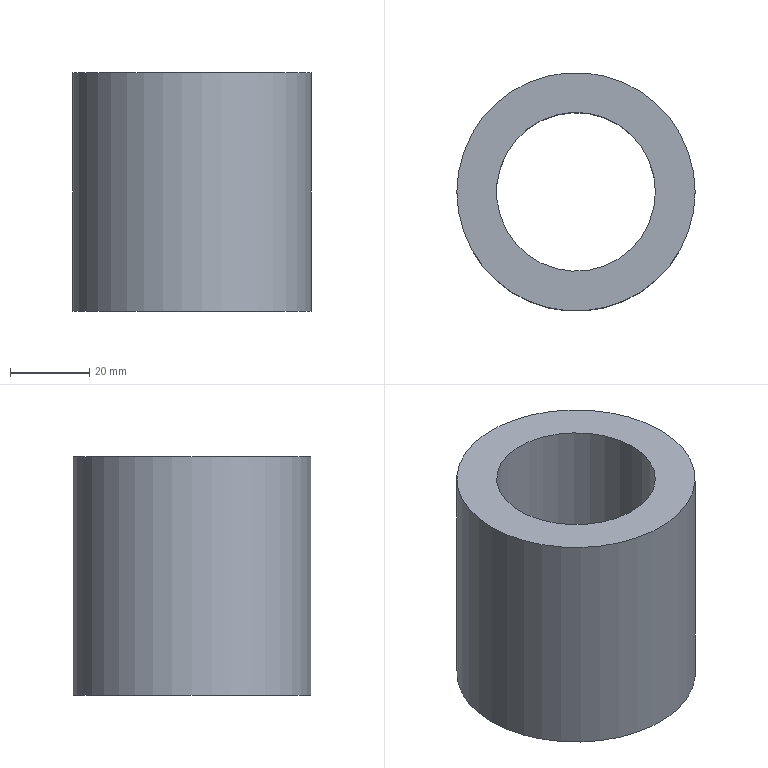Part | NX | features solid 2 | 1 solid | 4 faces | box 60 x 60 x 60 mm | volume 94248 mm3 | cylinder 2 | plane 2 | commonest cylinder face diameters 40 x1 60 x1
STEP:
#1=CARTESIAN_POINT('',(215.,25.,30.));
#2=VERTEX_POINT('',#1);
#3=CARTESIAN_POINT('',(195.,25.,30.));
#4=DIRECTION('',(0.,0.,-1.));
#5=DIRECTION('',(1.,0.,0.));
#6=AXIS2_PLACEMENT_3D('',#3,#4,#5);
#7=CIRCLE('',#6,20.);
#8=EDGE_CURVE('',#2,#2,#7,.T.);
#9=ORIENTED_EDGE('',*,*,#8,.T.);
#10=EDGE_LOOP('',(#9));
#11=FACE_BOUND('',#10,.T.);
#12=CARTESIAN_POINT('',(215.,25.,90.));
#13=VERTEX_POINT('',#12);
#14=CARTESIAN_POINT('',(195.,25.,90.));
#15=DIRECTION('',(0.,0.,-1.));
#16=DIRECTION('',(1.,0.,0.));
#17=AXIS2_PLACEMENT_3D('',#14,#15,#16);
#18=CIRCLE('',#17,20.);
#19=EDGE_CURVE('',#13,#13,#18,.T.);
#20=ORIENTED_EDGE('',*,*,#19,.F.);
#21=EDGE_LOOP('',(#20));
#22=FACE_BOUND('',#21,.T.);
#23=CARTESIAN_POINT('',(195.,25.,30.));
#24=DIRECTION('',(0.,0.,1.));
#25=DIRECTION('',(-1.,0.,0.));
#26=AXIS2_PLACEMENT_3D('',#23,#24,#25);
#27=CYLINDRICAL_SURFACE('',#26,20.);
#28=ADVANCED_FACE('',(#11,#22),#27,.F.);
#29=CARTESIAN_POINT('',(225.,25.,30.));
#30=VERTEX_POINT('',#29);
#31=CARTESIAN_POINT('',(195.,25.,30.));
#32=DIRECTION('',(0.,0.,-1.));
#33=DIRECTION('',(1.,0.,0.));
#34=AXIS2_PLACEMENT_3D('',#31,#32,#33);
#35=CIRCLE('',#34,30.);
#36=EDGE_CURVE('',#30,#30,#35,.T.);
#37=ORIENTED_EDGE('',*,*,#36,.F.);
#38=EDGE_LOOP('',(#37));
#39=FACE_BOUND('',#38,.T.);
#40=CARTESIAN_POINT('',(225.,25.,90.));
#41=VERTEX_POINT('',#40);
#42=CARTESIAN_POINT('',(195.,25.,90.));
#43=DIRECTION('',(0.,0.,-1.));
#44=DIRECTION('',(1.,0.,0.));
#45=AXIS2_PLACEMENT_3D('',#42,#43,#44);
#46=CIRCLE('',#45,30.);
#47=EDGE_CURVE('',#41,#41,#46,.T.);
#48=ORIENTED_EDGE('',*,*,#47,.T.);
#49=EDGE_LOOP('',(#48));
#50=FACE_BOUND('',#49,.T.);
#51=CARTESIAN_POINT('',(195.,25.,30.));
#52=DIRECTION('',(0.,0.,1.));
#53=DIRECTION('',(-1.,0.,0.));
#54=AXIS2_PLACEMENT_3D('',#51,#52,#53);
#55=CYLINDRICAL_SURFACE('',#54,30.);
#56=ADVANCED_FACE('',(#39,#50),#55,.T.);
#57=ORIENTED_EDGE('',*,*,#8,.F.);
#58=EDGE_LOOP('',(#57));
#59=FACE_BOUND('',#58,.T.);
#60=ORIENTED_EDGE('',*,*,#36,.T.);
#61=EDGE_LOOP('',(#60));
#62=FACE_BOUND('',#61,.T.);
#63=CARTESIAN_POINT('',(195.,25.,30.));
#64=DIRECTION('',(0.,0.,-1.));
#65=DIRECTION('',(1.,0.,0.));
#66=AXIS2_PLACEMENT_3D('',#63,#64,#65);
#67=PLANE('',#66);
#68=ADVANCED_FACE('',(#59,#62),#67,.T.);
#69=ORIENTED_EDGE('',*,*,#19,.T.);
#70=EDGE_LOOP('',(#69));
#71=FACE_BOUND('',#70,.T.);
#72=ORIENTED_EDGE('',*,*,#47,.F.);
#73=EDGE_LOOP('',(#72));
#74=FACE_BOUND('',#73,.T.);
#75=CARTESIAN_POINT('',(195.,25.,90.));
#76=DIRECTION('',(0.,0.,-1.));
#77=DIRECTION('',(1.,0.,0.));
#78=AXIS2_PLACEMENT_3D('',#75,#76,#77);
#79=PLANE('',#78);
#80=ADVANCED_FACE('',(#71,#74),#79,.F.);
#81=CLOSED_SHELL('',(#28,#56,#68,#80));
#82=MANIFOLD_SOLID_BREP('',#81);
#83=(LENGTH_UNIT()NAMED_UNIT(*)SI_UNIT(.MILLI.,.METRE.));
#84=UNCERTAINTY_MEASURE_WITH_UNIT(LENGTH_MEASURE(0.00001),#83,'','');
#85=(NAMED_UNIT(*)PLANE_ANGLE_UNIT()SI_UNIT($,.RADIAN.));
#86=(NAMED_UNIT(*)SI_UNIT($,.STERADIAN.)SOLID_ANGLE_UNIT());
#87=(GEOMETRIC_REPRESENTATION_CONTEXT(3)GLOBAL_UNCERTAINTY_ASSIGNED_CONTEXT((#84))GLOBAL_UNIT_ASSIGNED_CONTEXT((#83,#85,#86))REPRESENTATION_CONTEXT('',''));
#88=ADVANCED_BREP_SHAPE_REPRESENTATION('',(#82),#87);